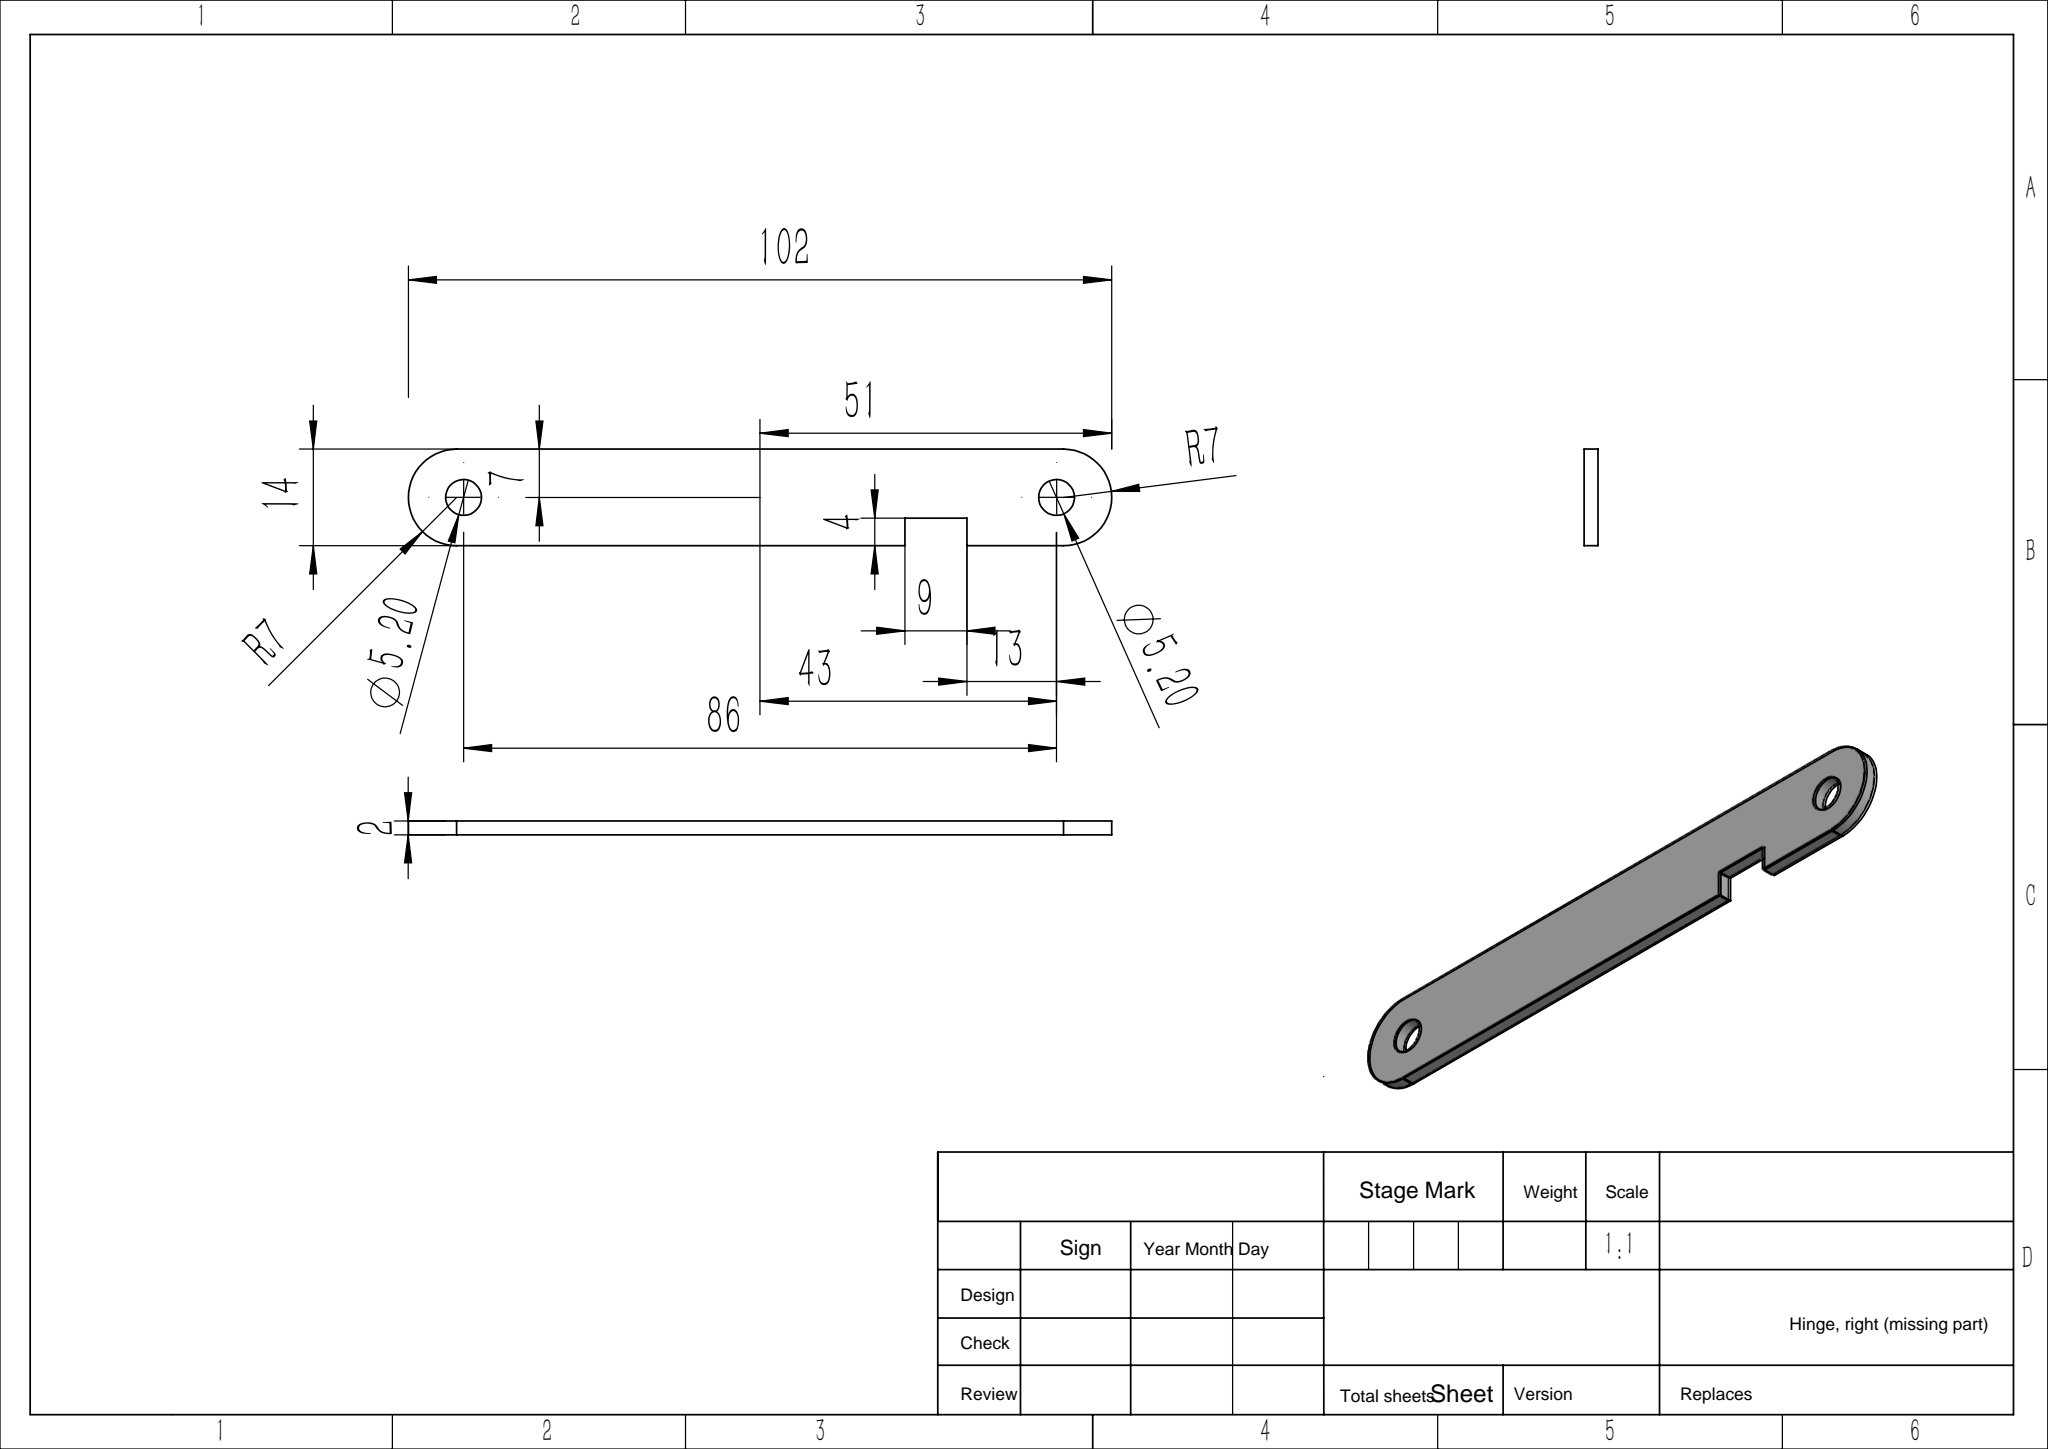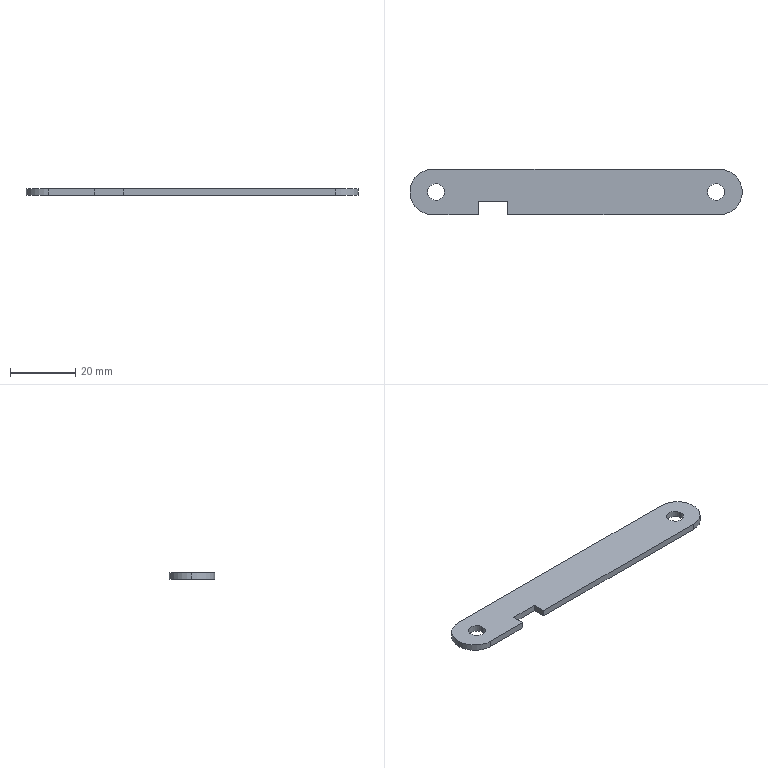Part | SolidWorks | features MirrorStock 1 | 1 solid | 15 faces | box 102 x 14 x 2 mm | volume 2615 mm3 | plane 8 | cylinder 7 | commonest cylinder face diameters 5.2 x4 14 x3
STEP:
#1=CARTESIAN_POINT('',(45.6,0.,-2.));
#2=VERTEX_POINT('',#1);
#3=CARTESIAN_POINT('',(40.4,0.,-2.));
#4=VERTEX_POINT('',#3);
#5=CARTESIAN_POINT('',(43.,0.,-2.));
#6=DIRECTION('',(0.,0.,1.));
#7=DIRECTION('',(1.,0.,0.));
#8=AXIS2_PLACEMENT_3D('',#5,#6,#7);
#9=CIRCLE('',#8,2.6);
#10=EDGE_CURVE('',#2,#4,#9,.T.);
#11=ORIENTED_EDGE('',*,*,#10,.F.);
#12=CARTESIAN_POINT('',(45.6,0.,0.));
#13=VERTEX_POINT('',#12);
#14=CARTESIAN_POINT('',(45.6,0.,-2.));
#15=DIRECTION('',(0.,0.,1.));
#16=VECTOR('',#15,1000.);
#17=LINE('',#14,#16);
#18=EDGE_CURVE('',#2,#13,#17,.T.);
#19=ORIENTED_EDGE('',*,*,#18,.T.);
#20=CARTESIAN_POINT('',(40.4,0.,0.));
#21=VERTEX_POINT('',#20);
#22=CARTESIAN_POINT('',(43.,0.,0.));
#23=DIRECTION('',(0.,0.,1.));
#24=DIRECTION('',(1.,0.,0.));
#25=AXIS2_PLACEMENT_3D('',#22,#23,#24);
#26=CIRCLE('',#25,2.6);
#27=EDGE_CURVE('',#13,#21,#26,.T.);
#28=ORIENTED_EDGE('',*,*,#27,.T.);
#29=CARTESIAN_POINT('',(40.4,0.,-2.));
#30=DIRECTION('',(0.,0.,1.));
#31=VECTOR('',#30,1000.);
#32=LINE('',#29,#31);
#33=EDGE_CURVE('',#4,#21,#32,.T.);
#34=ORIENTED_EDGE('',*,*,#33,.F.);
#35=EDGE_LOOP('',(#11,#19,#28,#34));
#36=FACE_OUTER_BOUND('',#35,.T.);
#37=CARTESIAN_POINT('',(43.,0.,-2.));
#38=DIRECTION('',(0.,0.,1.));
#39=DIRECTION('',(-1.,0.,0.));
#40=AXIS2_PLACEMENT_3D('',#37,#38,#39);
#41=CYLINDRICAL_SURFACE('',#40,2.6);
#42=ADVANCED_FACE('',(#36),#41,.F.);
#43=CARTESIAN_POINT('',(-40.4,0.,-2.));
#44=VERTEX_POINT('',#43);
#45=CARTESIAN_POINT('',(-45.6,0.,-2.));
#46=VERTEX_POINT('',#45);
#47=CARTESIAN_POINT('',(-43.,0.,-2.));
#48=DIRECTION('',(0.,0.,1.));
#49=DIRECTION('',(1.,0.,0.));
#50=AXIS2_PLACEMENT_3D('',#47,#48,#49);
#51=CIRCLE('',#50,2.6);
#52=EDGE_CURVE('',#44,#46,#51,.T.);
#53=ORIENTED_EDGE('',*,*,#52,.F.);
#54=CARTESIAN_POINT('',(-40.4,0.,0.));
#55=VERTEX_POINT('',#54);
#56=CARTESIAN_POINT('',(-40.4,0.,-2.));
#57=DIRECTION('',(0.,0.,1.));
#58=VECTOR('',#57,1000.);
#59=LINE('',#56,#58);
#60=EDGE_CURVE('',#44,#55,#59,.T.);
#61=ORIENTED_EDGE('',*,*,#60,.T.);
#62=CARTESIAN_POINT('',(-45.6,0.,0.));
#63=VERTEX_POINT('',#62);
#64=CARTESIAN_POINT('',(-43.,0.,0.));
#65=DIRECTION('',(0.,0.,1.));
#66=DIRECTION('',(1.,0.,0.));
#67=AXIS2_PLACEMENT_3D('',#64,#65,#66);
#68=CIRCLE('',#67,2.6);
#69=EDGE_CURVE('',#55,#63,#68,.T.);
#70=ORIENTED_EDGE('',*,*,#69,.T.);
#71=CARTESIAN_POINT('',(-45.6,0.,-2.));
#72=DIRECTION('',(0.,0.,1.));
#73=VECTOR('',#72,1000.);
#74=LINE('',#71,#73);
#75=EDGE_CURVE('',#46,#63,#74,.T.);
#76=ORIENTED_EDGE('',*,*,#75,.F.);
#77=EDGE_LOOP('',(#53,#61,#70,#76));
#78=FACE_OUTER_BOUND('',#77,.T.);
#79=CARTESIAN_POINT('',(-43.,0.,-2.));
#80=DIRECTION('',(0.,0.,1.));
#81=DIRECTION('',(-1.,0.,0.));
#82=AXIS2_PLACEMENT_3D('',#79,#80,#81);
#83=CYLINDRICAL_SURFACE('',#82,2.6);
#84=ADVANCED_FACE('',(#78),#83,.F.);
#85=CARTESIAN_POINT('',(-44.,7.,-2.));
#86=VERTEX_POINT('',#85);
#87=CARTESIAN_POINT('',(-51.,0.,-2.));
#88=VERTEX_POINT('',#87);
#89=CARTESIAN_POINT('',(-44.,0.,-2.));
#90=DIRECTION('',(0.,0.,1.));
#91=DIRECTION('',(1.,0.,0.));
#92=AXIS2_PLACEMENT_3D('',#89,#90,#91);
#93=CIRCLE('',#92,7.);
#94=EDGE_CURVE('',#86,#88,#93,.T.);
#95=ORIENTED_EDGE('',*,*,#94,.T.);
#96=CARTESIAN_POINT('',(-51.,0.,0.));
#97=VERTEX_POINT('',#96);
#98=CARTESIAN_POINT('',(-51.,0.,-2.));
#99=DIRECTION('',(0.,0.,1.));
#100=VECTOR('',#99,1000.);
#101=LINE('',#98,#100);
#102=EDGE_CURVE('',#88,#97,#101,.T.);
#103=ORIENTED_EDGE('',*,*,#102,.T.);
#104=CARTESIAN_POINT('',(-44.,7.,0.));
#105=VERTEX_POINT('',#104);
#106=CARTESIAN_POINT('',(-44.,0.,0.));
#107=DIRECTION('',(0.,0.,1.));
#108=DIRECTION('',(1.,0.,0.));
#109=AXIS2_PLACEMENT_3D('',#106,#107,#108);
#110=CIRCLE('',#109,7.);
#111=EDGE_CURVE('',#105,#97,#110,.T.);
#112=ORIENTED_EDGE('',*,*,#111,.F.);
#113=CARTESIAN_POINT('',(-44.,7.,-2.));
#114=DIRECTION('',(0.,0.,1.));
#115=VECTOR('',#114,1000.);
#116=LINE('',#113,#115);
#117=EDGE_CURVE('',#86,#105,#116,.T.);
#118=ORIENTED_EDGE('',*,*,#117,.F.);
#119=EDGE_LOOP('',(#95,#103,#112,#118));
#120=FACE_OUTER_BOUND('',#119,.T.);
#121=CARTESIAN_POINT('',(-44.,0.,-2.));
#122=DIRECTION('',(0.,0.,1.));
#123=DIRECTION('',(-1.,0.,0.));
#124=AXIS2_PLACEMENT_3D('',#121,#122,#123);
#125=CYLINDRICAL_SURFACE('',#124,7.);
#126=ADVANCED_FACE('',(#120),#125,.T.);
#127=CARTESIAN_POINT('',(-43.,0.,-2.));
#128=DIRECTION('',(0.,0.,1.));
#129=DIRECTION('',(1.,0.,0.));
#130=AXIS2_PLACEMENT_3D('',#127,#128,#129);
#131=CIRCLE('',#130,2.6);
#132=EDGE_CURVE('',#46,#44,#131,.T.);
#133=ORIENTED_EDGE('',*,*,#132,.T.);
#134=ORIENTED_EDGE('',*,*,#52,.T.);
#135=EDGE_LOOP('',(#133,#134));
#136=FACE_BOUND('',#135,.T.);
#137=CARTESIAN_POINT('',(44.,-7.,-2.));
#138=VERTEX_POINT('',#137);
#139=CARTESIAN_POINT('',(44.,7.,-2.));
#140=VERTEX_POINT('',#139);
#141=CARTESIAN_POINT('',(44.,0.,-2.));
#142=DIRECTION('',(0.,0.,1.));
#143=DIRECTION('',(1.,0.,0.));
#144=AXIS2_PLACEMENT_3D('',#141,#142,#143);
#145=CIRCLE('',#144,7.);
#146=EDGE_CURVE('',#138,#140,#145,.T.);
#147=ORIENTED_EDGE('',*,*,#146,.F.);
#148=CARTESIAN_POINT('',(-21.,-7.,-2.));
#149=VERTEX_POINT('',#148);
#150=CARTESIAN_POINT('',(-21.,-7.,-2.));
#151=DIRECTION('',(1.,0.,0.));
#152=VECTOR('',#151,1000.);
#153=LINE('',#150,#152);
#154=EDGE_CURVE('',#149,#138,#153,.T.);
#155=ORIENTED_EDGE('',*,*,#154,.F.);
#156=CARTESIAN_POINT('',(-21.,-3.,-2.));
#157=VERTEX_POINT('',#156);
#158=CARTESIAN_POINT('',(-21.,-3.,-2.));
#159=DIRECTION('',(0.,-1.,0.));
#160=VECTOR('',#159,1000.);
#161=LINE('',#158,#160);
#162=EDGE_CURVE('',#157,#149,#161,.T.);
#163=ORIENTED_EDGE('',*,*,#162,.F.);
#164=CARTESIAN_POINT('',(-30.,-3.,-2.));
#165=VERTEX_POINT('',#164);
#166=CARTESIAN_POINT('',(-30.,-3.,-2.));
#167=DIRECTION('',(1.,0.,0.));
#168=VECTOR('',#167,1000.);
#169=LINE('',#166,#168);
#170=EDGE_CURVE('',#165,#157,#169,.T.);
#171=ORIENTED_EDGE('',*,*,#170,.F.);
#172=CARTESIAN_POINT('',(-30.,-7.,-2.));
#173=VERTEX_POINT('',#172);
#174=CARTESIAN_POINT('',(-30.,-7.,-2.));
#175=DIRECTION('',(0.,1.,0.));
#176=VECTOR('',#175,1000.);
#177=LINE('',#174,#176);
#178=EDGE_CURVE('',#173,#165,#177,.T.);
#179=ORIENTED_EDGE('',*,*,#178,.F.);
#180=CARTESIAN_POINT('',(-44.,-7.,-2.));
#181=VERTEX_POINT('',#180);
#182=CARTESIAN_POINT('',(-44.,-7.,-2.));
#183=DIRECTION('',(1.,0.,0.));
#184=VECTOR('',#183,1000.);
#185=LINE('',#182,#184);
#186=EDGE_CURVE('',#181,#173,#185,.T.);
#187=ORIENTED_EDGE('',*,*,#186,.F.);
#188=CARTESIAN_POINT('',(-44.,0.,-2.));
#189=DIRECTION('',(0.,0.,1.));
#190=DIRECTION('',(1.,0.,0.));
#191=AXIS2_PLACEMENT_3D('',#188,#189,#190);
#192=CIRCLE('',#191,7.);
#193=EDGE_CURVE('',#88,#181,#192,.T.);
#194=ORIENTED_EDGE('',*,*,#193,.F.);
#195=ORIENTED_EDGE('',*,*,#94,.F.);
#196=CARTESIAN_POINT('',(-44.,7.,-2.));
#197=DIRECTION('',(-1.,0.,0.));
#198=VECTOR('',#197,1000.);
#199=LINE('',#196,#198);
#200=EDGE_CURVE('',#140,#86,#199,.T.);
#201=ORIENTED_EDGE('',*,*,#200,.F.);
#202=EDGE_LOOP('',(#147,#155,#163,#171,#179,#187,#194,#195,#201));
#203=FACE_OUTER_BOUND('',#202,.T.);
#204=CARTESIAN_POINT('',(43.,0.,-2.));
#205=DIRECTION('',(0.,0.,1.));
#206=DIRECTION('',(1.,0.,0.));
#207=AXIS2_PLACEMENT_3D('',#204,#205,#206);
#208=CIRCLE('',#207,2.6);
#209=EDGE_CURVE('',#4,#2,#208,.T.);
#210=ORIENTED_EDGE('',*,*,#209,.T.);
#211=ORIENTED_EDGE('',*,*,#10,.T.);
#212=EDGE_LOOP('',(#210,#211));
#213=FACE_BOUND('',#212,.T.);
#214=CARTESIAN_POINT('',(44.,0.,-2.));
#215=DIRECTION('',(0.,0.,-1.));
#216=DIRECTION('',(1.,0.,0.));
#217=AXIS2_PLACEMENT_3D('',#214,#215,#216);
#218=PLANE('',#217);
#219=ADVANCED_FACE('',(#136,#203,#213),#218,.T.);
#220=CARTESIAN_POINT('',(-43.,0.,0.));
#221=DIRECTION('',(0.,0.,1.));
#222=DIRECTION('',(1.,0.,0.));
#223=AXIS2_PLACEMENT_3D('',#220,#221,#222);
#224=CIRCLE('',#223,2.6);
#225=EDGE_CURVE('',#63,#55,#224,.T.);
#226=ORIENTED_EDGE('',*,*,#225,.F.);
#227=ORIENTED_EDGE('',*,*,#69,.F.);
#228=EDGE_LOOP('',(#226,#227));
#229=FACE_BOUND('',#228,.T.);
#230=CARTESIAN_POINT('',(44.,-7.,0.));
#231=VERTEX_POINT('',#230);
#232=CARTESIAN_POINT('',(44.,7.,0.));
#233=VERTEX_POINT('',#232);
#234=CARTESIAN_POINT('',(44.,0.,0.));
#235=DIRECTION('',(0.,0.,1.));
#236=DIRECTION('',(1.,0.,0.));
#237=AXIS2_PLACEMENT_3D('',#234,#235,#236);
#238=CIRCLE('',#237,7.);
#239=EDGE_CURVE('',#231,#233,#238,.T.);
#240=ORIENTED_EDGE('',*,*,#239,.T.);
#241=CARTESIAN_POINT('',(-44.,7.,0.));
#242=DIRECTION('',(-1.,0.,0.));
#243=VECTOR('',#242,1000.);
#244=LINE('',#241,#243);
#245=EDGE_CURVE('',#233,#105,#244,.T.);
#246=ORIENTED_EDGE('',*,*,#245,.T.);
#247=ORIENTED_EDGE('',*,*,#111,.T.);
#248=CARTESIAN_POINT('',(-44.,-7.,0.));
#249=VERTEX_POINT('',#248);
#250=CARTESIAN_POINT('',(-44.,0.,0.));
#251=DIRECTION('',(0.,0.,1.));
#252=DIRECTION('',(1.,0.,0.));
#253=AXIS2_PLACEMENT_3D('',#250,#251,#252);
#254=CIRCLE('',#253,7.);
#255=EDGE_CURVE('',#97,#249,#254,.T.);
#256=ORIENTED_EDGE('',*,*,#255,.T.);
#257=CARTESIAN_POINT('',(-30.,-7.,0.));
#258=VERTEX_POINT('',#257);
#259=CARTESIAN_POINT('',(-44.,-7.,0.));
#260=DIRECTION('',(1.,0.,0.));
#261=VECTOR('',#260,1000.);
#262=LINE('',#259,#261);
#263=EDGE_CURVE('',#249,#258,#262,.T.);
#264=ORIENTED_EDGE('',*,*,#263,.T.);
#265=CARTESIAN_POINT('',(-30.,-3.,0.));
#266=VERTEX_POINT('',#265);
#267=CARTESIAN_POINT('',(-30.,-7.,0.));
#268=DIRECTION('',(0.,1.,0.));
#269=VECTOR('',#268,1000.);
#270=LINE('',#267,#269);
#271=EDGE_CURVE('',#258,#266,#270,.T.);
#272=ORIENTED_EDGE('',*,*,#271,.T.);
#273=CARTESIAN_POINT('',(-21.,-3.,0.));
#274=VERTEX_POINT('',#273);
#275=CARTESIAN_POINT('',(-30.,-3.,0.));
#276=DIRECTION('',(1.,0.,0.));
#277=VECTOR('',#276,1000.);
#278=LINE('',#275,#277);
#279=EDGE_CURVE('',#266,#274,#278,.T.);
#280=ORIENTED_EDGE('',*,*,#279,.T.);
#281=CARTESIAN_POINT('',(-21.,-7.,0.));
#282=VERTEX_POINT('',#281);
#283=CARTESIAN_POINT('',(-21.,-3.,0.));
#284=DIRECTION('',(0.,-1.,0.));
#285=VECTOR('',#284,1000.);
#286=LINE('',#283,#285);
#287=EDGE_CURVE('',#274,#282,#286,.T.);
#288=ORIENTED_EDGE('',*,*,#287,.T.);
#289=CARTESIAN_POINT('',(-21.,-7.,0.));
#290=DIRECTION('',(1.,0.,0.));
#291=VECTOR('',#290,1000.);
#292=LINE('',#289,#291);
#293=EDGE_CURVE('',#282,#231,#292,.T.);
#294=ORIENTED_EDGE('',*,*,#293,.T.);
#295=EDGE_LOOP('',(#240,#246,#247,#256,#264,#272,#280,#288,#294));
#296=FACE_OUTER_BOUND('',#295,.T.);
#297=CARTESIAN_POINT('',(43.,0.,0.));
#298=DIRECTION('',(0.,0.,1.));
#299=DIRECTION('',(1.,0.,0.));
#300=AXIS2_PLACEMENT_3D('',#297,#298,#299);
#301=CIRCLE('',#300,2.6);
#302=EDGE_CURVE('',#21,#13,#301,.T.);
#303=ORIENTED_EDGE('',*,*,#302,.F.);
#304=ORIENTED_EDGE('',*,*,#27,.F.);
#305=EDGE_LOOP('',(#303,#304));
#306=FACE_BOUND('',#305,.T.);
#307=CARTESIAN_POINT('',(44.,0.,0.));
#308=DIRECTION('',(0.,0.,-1.));
#309=DIRECTION('',(1.,0.,0.));
#310=AXIS2_PLACEMENT_3D('',#307,#308,#309);
#311=PLANE('',#310);
#312=ADVANCED_FACE('',(#229,#296,#306),#311,.F.);
#313=ORIENTED_EDGE('',*,*,#239,.F.);
#314=CARTESIAN_POINT('',(44.,-7.,-2.));
#315=DIRECTION('',(0.,0.,1.));
#316=VECTOR('',#315,1000.);
#317=LINE('',#314,#316);
#318=EDGE_CURVE('',#138,#231,#317,.T.);
#319=ORIENTED_EDGE('',*,*,#318,.F.);
#320=ORIENTED_EDGE('',*,*,#146,.T.);
#321=CARTESIAN_POINT('',(44.,7.,-2.));
#322=DIRECTION('',(0.,0.,1.));
#323=VECTOR('',#322,1000.);
#324=LINE('',#321,#323);
#325=EDGE_CURVE('',#140,#233,#324,.T.);
#326=ORIENTED_EDGE('',*,*,#325,.T.);
#327=EDGE_LOOP('',(#313,#319,#320,#326));
#328=FACE_OUTER_BOUND('',#327,.T.);
#329=CARTESIAN_POINT('',(44.,0.,-2.));
#330=DIRECTION('',(0.,0.,1.));
#331=DIRECTION('',(-1.,0.,0.));
#332=AXIS2_PLACEMENT_3D('',#329,#330,#331);
#333=CYLINDRICAL_SURFACE('',#332,7.);
#334=ADVANCED_FACE('',(#328),#333,.T.);
#335=ORIENTED_EDGE('',*,*,#245,.F.);
#336=ORIENTED_EDGE('',*,*,#325,.F.);
#337=ORIENTED_EDGE('',*,*,#200,.T.);
#338=ORIENTED_EDGE('',*,*,#117,.T.);
#339=EDGE_LOOP('',(#335,#336,#337,#338));
#340=FACE_OUTER_BOUND('',#339,.T.);
#341=CARTESIAN_POINT('',(-44.,7.,-2.));
#342=DIRECTION('',(0.,-1.,0.));
#343=DIRECTION('',(0.,0.,1.));
#344=AXIS2_PLACEMENT_3D('',#341,#342,#343);
#345=PLANE('',#344);
#346=ADVANCED_FACE('',(#340),#345,.F.);
#347=ORIENTED_EDGE('',*,*,#102,.F.);
#348=ORIENTED_EDGE('',*,*,#193,.T.);
#349=CARTESIAN_POINT('',(-44.,-7.,-2.));
#350=DIRECTION('',(0.,0.,1.));
#351=VECTOR('',#350,1000.);
#352=LINE('',#349,#351);
#353=EDGE_CURVE('',#181,#249,#352,.T.);
#354=ORIENTED_EDGE('',*,*,#353,.T.);
#355=ORIENTED_EDGE('',*,*,#255,.F.);
#356=EDGE_LOOP('',(#347,#348,#354,#355));
#357=FACE_OUTER_BOUND('',#356,.T.);
#358=CARTESIAN_POINT('',(-44.,0.,-2.));
#359=DIRECTION('',(0.,0.,1.));
#360=DIRECTION('',(-1.,0.,0.));
#361=AXIS2_PLACEMENT_3D('',#358,#359,#360);
#362=CYLINDRICAL_SURFACE('',#361,7.);
#363=ADVANCED_FACE('',(#357),#362,.T.);
#364=ORIENTED_EDGE('',*,*,#263,.F.);
#365=ORIENTED_EDGE('',*,*,#353,.F.);
#366=ORIENTED_EDGE('',*,*,#186,.T.);
#367=CARTESIAN_POINT('',(-30.,-7.,-2.));
#368=DIRECTION('',(0.,0.,1.));
#369=VECTOR('',#368,1000.);
#370=LINE('',#367,#369);
#371=EDGE_CURVE('',#173,#258,#370,.T.);
#372=ORIENTED_EDGE('',*,*,#371,.T.);
#373=EDGE_LOOP('',(#364,#365,#366,#372));
#374=FACE_OUTER_BOUND('',#373,.T.);
#375=CARTESIAN_POINT('',(-44.,-7.,-2.));
#376=DIRECTION('',(0.,1.,0.));
#377=DIRECTION('',(0.,0.,-1.));
#378=AXIS2_PLACEMENT_3D('',#375,#376,#377);
#379=PLANE('',#378);
#380=ADVANCED_FACE('',(#374),#379,.F.);
#381=ORIENTED_EDGE('',*,*,#271,.F.);
#382=ORIENTED_EDGE('',*,*,#371,.F.);
#383=ORIENTED_EDGE('',*,*,#178,.T.);
#384=CARTESIAN_POINT('',(-30.,-3.,-2.));
#385=DIRECTION('',(0.,0.,1.));
#386=VECTOR('',#385,1000.);
#387=LINE('',#384,#386);
#388=EDGE_CURVE('',#165,#266,#387,.T.);
#389=ORIENTED_EDGE('',*,*,#388,.T.);
#390=EDGE_LOOP('',(#381,#382,#383,#389));
#391=FACE_OUTER_BOUND('',#390,.T.);
#392=CARTESIAN_POINT('',(-30.,-7.,-2.));
#393=DIRECTION('',(-1.,0.,0.));
#394=DIRECTION('',(0.,-1.,0.));
#395=AXIS2_PLACEMENT_3D('',#392,#393,#394);
#396=PLANE('',#395);
#397=ADVANCED_FACE('',(#391),#396,.F.);
#398=ORIENTED_EDGE('',*,*,#279,.F.);
#399=ORIENTED_EDGE('',*,*,#388,.F.);
#400=ORIENTED_EDGE('',*,*,#170,.T.);
#401=CARTESIAN_POINT('',(-21.,-3.,-2.));
#402=DIRECTION('',(0.,0.,1.));
#403=VECTOR('',#402,1000.);
#404=LINE('',#401,#403);
#405=EDGE_CURVE('',#157,#274,#404,.T.);
#406=ORIENTED_EDGE('',*,*,#405,.T.);
#407=EDGE_LOOP('',(#398,#399,#400,#406));
#408=FACE_OUTER_BOUND('',#407,.T.);
#409=CARTESIAN_POINT('',(-30.,-3.,-2.));
#410=DIRECTION('',(0.,1.,0.));
#411=DIRECTION('',(0.,0.,-1.));
#412=AXIS2_PLACEMENT_3D('',#409,#410,#411);
#413=PLANE('',#412);
#414=ADVANCED_FACE('',(#408),#413,.F.);
#415=ORIENTED_EDGE('',*,*,#287,.F.);
#416=ORIENTED_EDGE('',*,*,#405,.F.);
#417=ORIENTED_EDGE('',*,*,#162,.T.);
#418=CARTESIAN_POINT('',(-21.,-7.,-2.));
#419=DIRECTION('',(0.,0.,1.));
#420=VECTOR('',#419,1000.);
#421=LINE('',#418,#420);
#422=EDGE_CURVE('',#149,#282,#421,.T.);
#423=ORIENTED_EDGE('',*,*,#422,.T.);
#424=EDGE_LOOP('',(#415,#416,#417,#423));
#425=FACE_OUTER_BOUND('',#424,.T.);
#426=CARTESIAN_POINT('',(-21.,-3.,-2.));
#427=DIRECTION('',(1.,0.,0.));
#428=DIRECTION('',(0.,0.,1.));
#429=AXIS2_PLACEMENT_3D('',#426,#427,#428);
#430=PLANE('',#429);
#431=ADVANCED_FACE('',(#425),#430,.F.);
#432=ORIENTED_EDGE('',*,*,#293,.F.);
#433=ORIENTED_EDGE('',*,*,#422,.F.);
#434=ORIENTED_EDGE('',*,*,#154,.T.);
#435=ORIENTED_EDGE('',*,*,#318,.T.);
#436=EDGE_LOOP('',(#432,#433,#434,#435));
#437=FACE_OUTER_BOUND('',#436,.T.);
#438=CARTESIAN_POINT('',(-21.,-7.,-2.));
#439=DIRECTION('',(0.,1.,0.));
#440=DIRECTION('',(0.,0.,-1.));
#441=AXIS2_PLACEMENT_3D('',#438,#439,#440);
#442=PLANE('',#441);
#443=ADVANCED_FACE('',(#437),#442,.F.);
#444=ORIENTED_EDGE('',*,*,#60,.F.);
#445=ORIENTED_EDGE('',*,*,#132,.F.);
#446=ORIENTED_EDGE('',*,*,#75,.T.);
#447=ORIENTED_EDGE('',*,*,#225,.T.);
#448=EDGE_LOOP('',(#444,#445,#446,#447));
#449=FACE_OUTER_BOUND('',#448,.T.);
#450=CARTESIAN_POINT('',(-43.,0.,-2.));
#451=DIRECTION('',(0.,0.,1.));
#452=DIRECTION('',(-1.,0.,0.));
#453=AXIS2_PLACEMENT_3D('',#450,#451,#452);
#454=CYLINDRICAL_SURFACE('',#453,2.6);
#455=ADVANCED_FACE('',(#449),#454,.F.);
#456=ORIENTED_EDGE('',*,*,#18,.F.);
#457=ORIENTED_EDGE('',*,*,#209,.F.);
#458=ORIENTED_EDGE('',*,*,#33,.T.);
#459=ORIENTED_EDGE('',*,*,#302,.T.);
#460=EDGE_LOOP('',(#456,#457,#458,#459));
#461=FACE_OUTER_BOUND('',#460,.T.);
#462=CARTESIAN_POINT('',(43.,0.,-2.));
#463=DIRECTION('',(0.,0.,1.));
#464=DIRECTION('',(-1.,0.,0.));
#465=AXIS2_PLACEMENT_3D('',#462,#463,#464);
#466=CYLINDRICAL_SURFACE('',#465,2.6);
#467=ADVANCED_FACE('',(#461),#466,.F.);
#468=CLOSED_SHELL('',(#42,#84,#126,#219,#312,#334,#346,#363,#380,#397,#414,#431,#443,#455,#467));
#469=MANIFOLD_SOLID_BREP('',#468);
#470=CARTESIAN_POINT('',(0.,0.,0.));
#471=DIRECTION('',(0.,0.,1.));
#472=DIRECTION('',(1.,0.,0.));
#473=AXIS2_PLACEMENT_3D('',#470,#471,#472);
#474=(LENGTH_UNIT()NAMED_UNIT(*)SI_UNIT(.MILLI.,.METRE.));
#475=UNCERTAINTY_MEASURE_WITH_UNIT(LENGTH_MEASURE(0.00001),#474,'','');
#476=(NAMED_UNIT(*)PLANE_ANGLE_UNIT()SI_UNIT($,.RADIAN.));
#477=(NAMED_UNIT(*)SI_UNIT($,.STERADIAN.)SOLID_ANGLE_UNIT());
#478=(GEOMETRIC_REPRESENTATION_CONTEXT(3)GLOBAL_UNCERTAINTY_ASSIGNED_CONTEXT((#475))GLOBAL_UNIT_ASSIGNED_CONTEXT((#474,#476,#477))REPRESENTATION_CONTEXT('',''));
#479=ADVANCED_BREP_SHAPE_REPRESENTATION('',(#469,#473),#478);